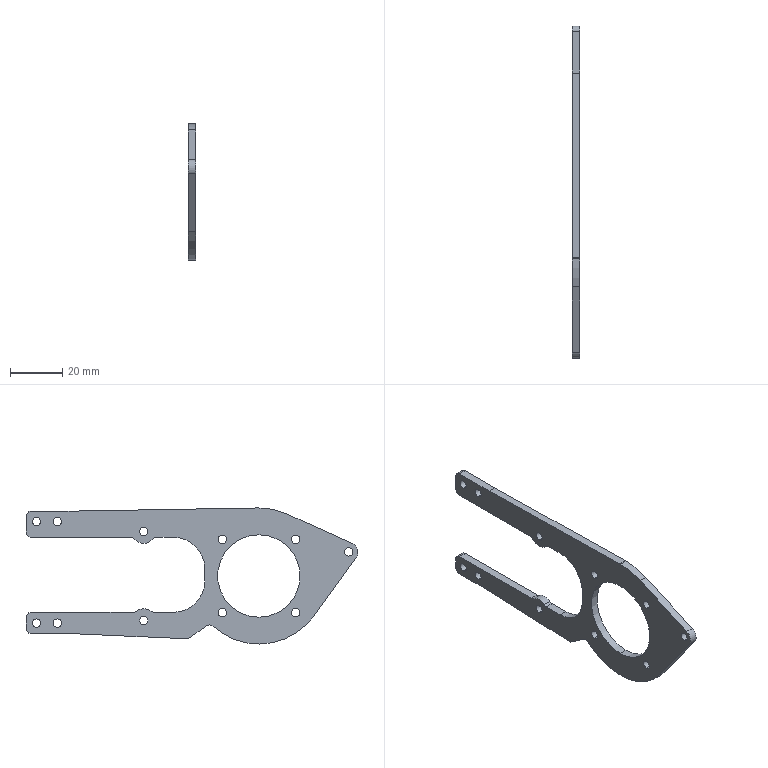Part | SolidWorks | features ICE 3, Fillet 2, Extrusion 1 | 1 solid | 62 faces | box 3 x 126.828 x 52 mm | volume 8428 mm3 | cylinder 46 | plane 16 | commonest cylinder face diameters 3.2 x22 4 x13 9 x3 52 x3 24 x2 31.5 x2